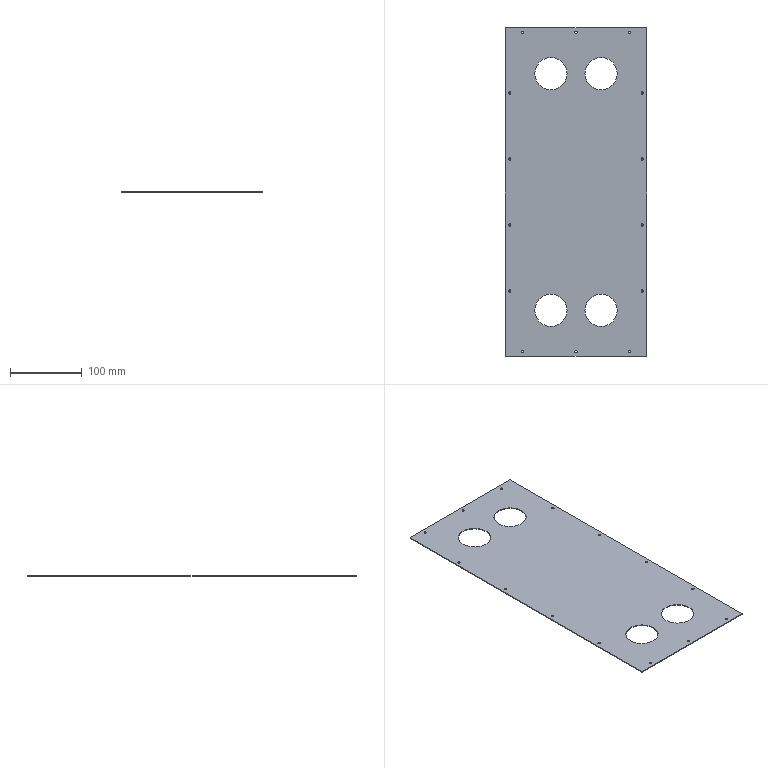Part | STEP file | TL42B-88D-3-plate heat exchanger 3 | 1 solid | 46 faces | box 198 x 458 x 1 mm | volume 84209 mm3 | cylinder 40 | plane 6 | commonest cylinder face diameters 3.2 x28 45 x8 2 x4